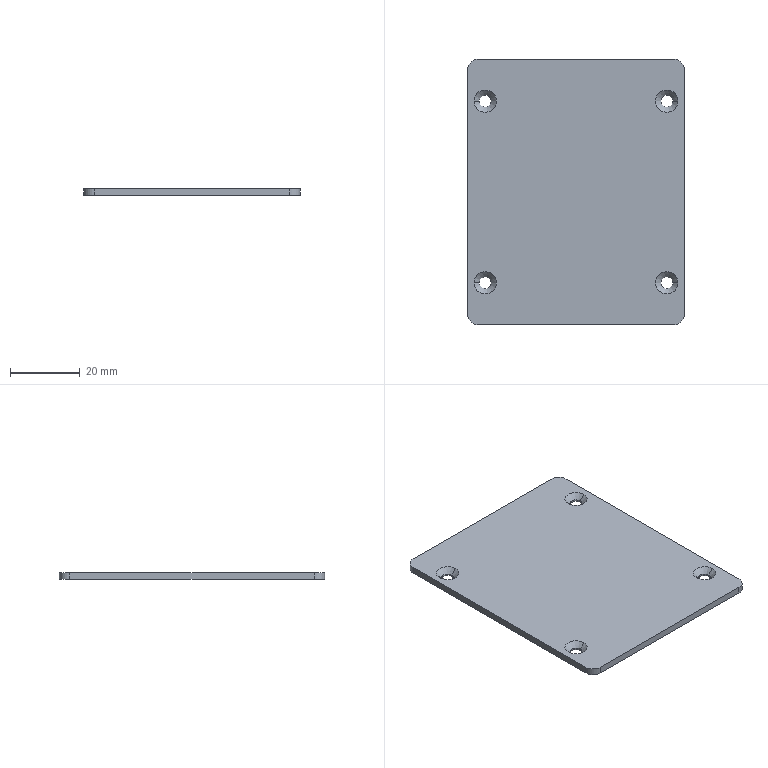Part | STEP file | 复件 FHB175-033^FHB175S-PRW-P40(马达RightUpper折-400W伺服电机) | 1 solid | 26 faces | box 62 x 76 x 2 mm | volume 9274 mm3 | cylinder 12 | cone 8 | plane 6 | commonest cylinder face diameters 3.4 x8 6 x4
STEP:
#1=CARTESIAN_POINT('',(-20.307,6.451,0.));
#2=VERTEX_POINT('',#1);
#3=CARTESIAN_POINT('',(-16.907,6.451,0.));
#4=VERTEX_POINT('',#3);
#5=CARTESIAN_POINT('',(-18.607,6.451,0.));
#6=DIRECTION('',(0.,0.,1.));
#7=DIRECTION('',(1.,0.,0.));
#8=AXIS2_PLACEMENT_3D('',#5,#6,#7);
#9=CIRCLE('',#8,1.7);
#10=EDGE_CURVE('',#2,#4,#9,.T.);
#11=ORIENTED_EDGE('',*,*,#10,.F.);
#12=CARTESIAN_POINT('',(-20.307,6.451,0.5));
#13=VERTEX_POINT('',#12);
#14=CARTESIAN_POINT('',(-20.307,6.451,2.));
#15=DIRECTION('',(0.,0.,1.));
#16=VECTOR('',#15,1000.);
#17=LINE('',#14,#16);
#18=EDGE_CURVE('',#2,#13,#17,.T.);
#19=ORIENTED_EDGE('',*,*,#18,.T.);
#20=CARTESIAN_POINT('',(-16.907,6.451,0.5));
#21=VERTEX_POINT('',#20);
#22=CARTESIAN_POINT('',(-18.607,6.451,0.5));
#23=DIRECTION('',(0.,0.,-1.));
#24=DIRECTION('',(1.,0.,0.));
#25=AXIS2_PLACEMENT_3D('',#22,#23,#24);
#26=CIRCLE('',#25,1.7);
#27=EDGE_CURVE('',#21,#13,#26,.T.);
#28=ORIENTED_EDGE('',*,*,#27,.F.);
#29=CARTESIAN_POINT('',(-16.907,6.451,2.));
#30=DIRECTION('',(0.,0.,1.));
#31=VECTOR('',#30,1000.);
#32=LINE('',#29,#31);
#33=EDGE_CURVE('',#4,#21,#32,.T.);
#34=ORIENTED_EDGE('',*,*,#33,.F.);
#35=EDGE_LOOP('',(#11,#19,#28,#34));
#36=FACE_OUTER_BOUND('',#35,.T.);
#37=CARTESIAN_POINT('',(-18.607,6.451,2.));
#38=DIRECTION('',(0.,0.,1.));
#39=DIRECTION('',(1.,0.,0.));
#40=AXIS2_PLACEMENT_3D('',#37,#38,#39);
#41=CYLINDRICAL_SURFACE('',#40,1.7);
#42=ADVANCED_FACE('',(#36),#41,.F.);
#43=CARTESIAN_POINT('',(-20.307,58.451,0.));
#44=VERTEX_POINT('',#43);
#45=CARTESIAN_POINT('',(-16.907,58.451,0.));
#46=VERTEX_POINT('',#45);
#47=CARTESIAN_POINT('',(-18.607,58.451,0.));
#48=DIRECTION('',(0.,0.,1.));
#49=DIRECTION('',(1.,0.,0.));
#50=AXIS2_PLACEMENT_3D('',#47,#48,#49);
#51=CIRCLE('',#50,1.7);
#52=EDGE_CURVE('',#44,#46,#51,.T.);
#53=ORIENTED_EDGE('',*,*,#52,.F.);
#54=CARTESIAN_POINT('',(-20.307,58.451,0.5));
#55=VERTEX_POINT('',#54);
#56=CARTESIAN_POINT('',(-20.307,58.451,2.));
#57=DIRECTION('',(0.,0.,1.));
#58=VECTOR('',#57,1000.);
#59=LINE('',#56,#58);
#60=EDGE_CURVE('',#44,#55,#59,.T.);
#61=ORIENTED_EDGE('',*,*,#60,.T.);
#62=CARTESIAN_POINT('',(-16.907,58.451,0.5));
#63=VERTEX_POINT('',#62);
#64=CARTESIAN_POINT('',(-18.607,58.451,0.5));
#65=DIRECTION('',(0.,0.,-1.));
#66=DIRECTION('',(1.,0.,0.));
#67=AXIS2_PLACEMENT_3D('',#64,#65,#66);
#68=CIRCLE('',#67,1.7);
#69=EDGE_CURVE('',#63,#55,#68,.T.);
#70=ORIENTED_EDGE('',*,*,#69,.F.);
#71=CARTESIAN_POINT('',(-16.907,58.451,2.));
#72=DIRECTION('',(0.,0.,1.));
#73=VECTOR('',#72,1000.);
#74=LINE('',#71,#73);
#75=EDGE_CURVE('',#46,#63,#74,.T.);
#76=ORIENTED_EDGE('',*,*,#75,.F.);
#77=EDGE_LOOP('',(#53,#61,#70,#76));
#78=FACE_OUTER_BOUND('',#77,.T.);
#79=CARTESIAN_POINT('',(-18.607,58.451,2.));
#80=DIRECTION('',(0.,0.,1.));
#81=DIRECTION('',(1.,0.,0.));
#82=AXIS2_PLACEMENT_3D('',#79,#80,#81);
#83=CYLINDRICAL_SURFACE('',#82,1.7);
#84=ADVANCED_FACE('',(#78),#83,.F.);
#85=CARTESIAN_POINT('',(31.693,58.451,0.));
#86=VERTEX_POINT('',#85);
#87=CARTESIAN_POINT('',(35.093,58.451,0.));
#88=VERTEX_POINT('',#87);
#89=CARTESIAN_POINT('',(33.393,58.451,0.));
#90=DIRECTION('',(0.,0.,1.));
#91=DIRECTION('',(1.,0.,0.));
#92=AXIS2_PLACEMENT_3D('',#89,#90,#91);
#93=CIRCLE('',#92,1.7);
#94=EDGE_CURVE('',#86,#88,#93,.T.);
#95=ORIENTED_EDGE('',*,*,#94,.F.);
#96=CARTESIAN_POINT('',(31.693,58.451,0.5));
#97=VERTEX_POINT('',#96);
#98=CARTESIAN_POINT('',(31.693,58.451,2.));
#99=DIRECTION('',(0.,0.,1.));
#100=VECTOR('',#99,1000.);
#101=LINE('',#98,#100);
#102=EDGE_CURVE('',#86,#97,#101,.T.);
#103=ORIENTED_EDGE('',*,*,#102,.T.);
#104=CARTESIAN_POINT('',(35.093,58.451,0.5));
#105=VERTEX_POINT('',#104);
#106=CARTESIAN_POINT('',(33.393,58.451,0.5));
#107=DIRECTION('',(0.,0.,-1.));
#108=DIRECTION('',(1.,0.,0.));
#109=AXIS2_PLACEMENT_3D('',#106,#107,#108);
#110=CIRCLE('',#109,1.7);
#111=EDGE_CURVE('',#105,#97,#110,.T.);
#112=ORIENTED_EDGE('',*,*,#111,.F.);
#113=CARTESIAN_POINT('',(35.093,58.451,2.));
#114=DIRECTION('',(0.,0.,1.));
#115=VECTOR('',#114,1000.);
#116=LINE('',#113,#115);
#117=EDGE_CURVE('',#88,#105,#116,.T.);
#118=ORIENTED_EDGE('',*,*,#117,.F.);
#119=EDGE_LOOP('',(#95,#103,#112,#118));
#120=FACE_OUTER_BOUND('',#119,.T.);
#121=CARTESIAN_POINT('',(33.393,58.451,2.));
#122=DIRECTION('',(0.,0.,1.));
#123=DIRECTION('',(1.,0.,0.));
#124=AXIS2_PLACEMENT_3D('',#121,#122,#123);
#125=CYLINDRICAL_SURFACE('',#124,1.7);
#126=ADVANCED_FACE('',(#120),#125,.F.);
#127=CARTESIAN_POINT('',(31.693,6.451,0.));
#128=VERTEX_POINT('',#127);
#129=CARTESIAN_POINT('',(35.093,6.451,0.));
#130=VERTEX_POINT('',#129);
#131=CARTESIAN_POINT('',(33.393,6.451,0.));
#132=DIRECTION('',(0.,0.,1.));
#133=DIRECTION('',(1.,0.,0.));
#134=AXIS2_PLACEMENT_3D('',#131,#132,#133);
#135=CIRCLE('',#134,1.7);
#136=EDGE_CURVE('',#128,#130,#135,.T.);
#137=ORIENTED_EDGE('',*,*,#136,.F.);
#138=CARTESIAN_POINT('',(31.693,6.451,0.5));
#139=VERTEX_POINT('',#138);
#140=CARTESIAN_POINT('',(31.693,6.451,2.));
#141=DIRECTION('',(0.,0.,1.));
#142=VECTOR('',#141,1000.);
#143=LINE('',#140,#142);
#144=EDGE_CURVE('',#128,#139,#143,.T.);
#145=ORIENTED_EDGE('',*,*,#144,.T.);
#146=CARTESIAN_POINT('',(35.093,6.451,0.5));
#147=VERTEX_POINT('',#146);
#148=CARTESIAN_POINT('',(33.393,6.451,0.5));
#149=DIRECTION('',(0.,0.,-1.));
#150=DIRECTION('',(1.,0.,0.));
#151=AXIS2_PLACEMENT_3D('',#148,#149,#150);
#152=CIRCLE('',#151,1.7);
#153=EDGE_CURVE('',#147,#139,#152,.T.);
#154=ORIENTED_EDGE('',*,*,#153,.F.);
#155=CARTESIAN_POINT('',(35.093,6.451,2.));
#156=DIRECTION('',(0.,0.,1.));
#157=VECTOR('',#156,1000.);
#158=LINE('',#155,#157);
#159=EDGE_CURVE('',#130,#147,#158,.T.);
#160=ORIENTED_EDGE('',*,*,#159,.F.);
#161=EDGE_LOOP('',(#137,#145,#154,#160));
#162=FACE_OUTER_BOUND('',#161,.T.);
#163=CARTESIAN_POINT('',(33.393,6.451,2.));
#164=DIRECTION('',(0.,0.,1.));
#165=DIRECTION('',(1.,0.,0.));
#166=AXIS2_PLACEMENT_3D('',#163,#164,#165);
#167=CYLINDRICAL_SURFACE('',#166,1.7);
#168=ADVANCED_FACE('',(#162),#167,.F.);
#169=ORIENTED_EDGE('',*,*,#27,.T.);
#170=CARTESIAN_POINT('',(-21.807,6.451,2.));
#171=VERTEX_POINT('',#170);
#172=CARTESIAN_POINT('',(-21.807,6.451,2.));
#173=DIRECTION('',(-0.7071,0.,0.7071));
#174=VECTOR('',#173,1000.);
#175=LINE('',#172,#174);
#176=EDGE_CURVE('',#13,#171,#175,.T.);
#177=ORIENTED_EDGE('',*,*,#176,.T.);
#178=CARTESIAN_POINT('',(-15.407,6.451,2.));
#179=VERTEX_POINT('',#178);
#180=CARTESIAN_POINT('',(-18.607,6.451,2.));
#181=DIRECTION('',(0.,0.,1.));
#182=DIRECTION('',(1.,0.,0.));
#183=AXIS2_PLACEMENT_3D('',#180,#181,#182);
#184=CIRCLE('',#183,3.2);
#185=EDGE_CURVE('',#171,#179,#184,.T.);
#186=ORIENTED_EDGE('',*,*,#185,.T.);
#187=CARTESIAN_POINT('',(-15.407,6.451,2.));
#188=DIRECTION('',(0.7071,0.,0.7071));
#189=VECTOR('',#188,1000.);
#190=LINE('',#187,#189);
#191=EDGE_CURVE('',#21,#179,#190,.T.);
#192=ORIENTED_EDGE('',*,*,#191,.F.);
#193=EDGE_LOOP('',(#169,#177,#186,#192));
#194=FACE_OUTER_BOUND('',#193,.T.);
#195=CARTESIAN_POINT('',(-18.607,6.451,2.));
#196=DIRECTION('',(0.,0.,1.));
#197=DIRECTION('',(1.,0.,0.));
#198=AXIS2_PLACEMENT_3D('',#195,#196,#197);
#199=CONICAL_SURFACE('',#198,3.2,0.7854);
#200=ADVANCED_FACE('',(#194),#199,.F.);
#201=ORIENTED_EDGE('',*,*,#69,.T.);
#202=CARTESIAN_POINT('',(-21.807,58.451,2.));
#203=VERTEX_POINT('',#202);
#204=CARTESIAN_POINT('',(-21.807,58.451,2.));
#205=DIRECTION('',(-0.7071,0.,0.7071));
#206=VECTOR('',#205,1000.);
#207=LINE('',#204,#206);
#208=EDGE_CURVE('',#55,#203,#207,.T.);
#209=ORIENTED_EDGE('',*,*,#208,.T.);
#210=CARTESIAN_POINT('',(-15.407,58.451,2.));
#211=VERTEX_POINT('',#210);
#212=CARTESIAN_POINT('',(-18.607,58.451,2.));
#213=DIRECTION('',(0.,0.,1.));
#214=DIRECTION('',(1.,0.,0.));
#215=AXIS2_PLACEMENT_3D('',#212,#213,#214);
#216=CIRCLE('',#215,3.2);
#217=EDGE_CURVE('',#203,#211,#216,.T.);
#218=ORIENTED_EDGE('',*,*,#217,.T.);
#219=CARTESIAN_POINT('',(-15.407,58.451,2.));
#220=DIRECTION('',(0.7071,0.,0.7071));
#221=VECTOR('',#220,1000.);
#222=LINE('',#219,#221);
#223=EDGE_CURVE('',#63,#211,#222,.T.);
#224=ORIENTED_EDGE('',*,*,#223,.F.);
#225=EDGE_LOOP('',(#201,#209,#218,#224));
#226=FACE_OUTER_BOUND('',#225,.T.);
#227=CARTESIAN_POINT('',(-18.607,58.451,2.));
#228=DIRECTION('',(0.,0.,1.));
#229=DIRECTION('',(1.,0.,0.));
#230=AXIS2_PLACEMENT_3D('',#227,#228,#229);
#231=CONICAL_SURFACE('',#230,3.2,0.7854);
#232=ADVANCED_FACE('',(#226),#231,.F.);
#233=ORIENTED_EDGE('',*,*,#111,.T.);
#234=CARTESIAN_POINT('',(30.193,58.451,2.));
#235=VERTEX_POINT('',#234);
#236=CARTESIAN_POINT('',(30.193,58.451,2.));
#237=DIRECTION('',(-0.7071,0.,0.7071));
#238=VECTOR('',#237,1000.);
#239=LINE('',#236,#238);
#240=EDGE_CURVE('',#97,#235,#239,.T.);
#241=ORIENTED_EDGE('',*,*,#240,.T.);
#242=CARTESIAN_POINT('',(36.593,58.451,2.));
#243=VERTEX_POINT('',#242);
#244=CARTESIAN_POINT('',(33.393,58.451,2.));
#245=DIRECTION('',(0.,0.,1.));
#246=DIRECTION('',(1.,0.,0.));
#247=AXIS2_PLACEMENT_3D('',#244,#245,#246);
#248=CIRCLE('',#247,3.2);
#249=EDGE_CURVE('',#235,#243,#248,.T.);
#250=ORIENTED_EDGE('',*,*,#249,.T.);
#251=CARTESIAN_POINT('',(36.593,58.451,2.));
#252=DIRECTION('',(0.7071,0.,0.7071));
#253=VECTOR('',#252,1000.);
#254=LINE('',#251,#253);
#255=EDGE_CURVE('',#105,#243,#254,.T.);
#256=ORIENTED_EDGE('',*,*,#255,.F.);
#257=EDGE_LOOP('',(#233,#241,#250,#256));
#258=FACE_OUTER_BOUND('',#257,.T.);
#259=CARTESIAN_POINT('',(33.393,58.451,2.));
#260=DIRECTION('',(0.,0.,1.));
#261=DIRECTION('',(1.,0.,0.));
#262=AXIS2_PLACEMENT_3D('',#259,#260,#261);
#263=CONICAL_SURFACE('',#262,3.2,0.7854);
#264=ADVANCED_FACE('',(#258),#263,.F.);
#265=ORIENTED_EDGE('',*,*,#153,.T.);
#266=CARTESIAN_POINT('',(30.193,6.451,2.));
#267=VERTEX_POINT('',#266);
#268=CARTESIAN_POINT('',(30.193,6.451,2.));
#269=DIRECTION('',(-0.7071,0.,0.7071));
#270=VECTOR('',#269,1000.);
#271=LINE('',#268,#270);
#272=EDGE_CURVE('',#139,#267,#271,.T.);
#273=ORIENTED_EDGE('',*,*,#272,.T.);
#274=CARTESIAN_POINT('',(36.593,6.451,2.));
#275=VERTEX_POINT('',#274);
#276=CARTESIAN_POINT('',(33.393,6.451,2.));
#277=DIRECTION('',(0.,0.,1.));
#278=DIRECTION('',(1.,0.,0.));
#279=AXIS2_PLACEMENT_3D('',#276,#277,#278);
#280=CIRCLE('',#279,3.2);
#281=EDGE_CURVE('',#267,#275,#280,.T.);
#282=ORIENTED_EDGE('',*,*,#281,.T.);
#283=CARTESIAN_POINT('',(36.593,6.451,2.));
#284=DIRECTION('',(0.7071,0.,0.7071));
#285=VECTOR('',#284,1000.);
#286=LINE('',#283,#285);
#287=EDGE_CURVE('',#147,#275,#286,.T.);
#288=ORIENTED_EDGE('',*,*,#287,.F.);
#289=EDGE_LOOP('',(#265,#273,#282,#288));
#290=FACE_OUTER_BOUND('',#289,.T.);
#291=CARTESIAN_POINT('',(33.393,6.451,2.));
#292=DIRECTION('',(0.,0.,1.));
#293=DIRECTION('',(1.,0.,0.));
#294=AXIS2_PLACEMENT_3D('',#291,#292,#293);
#295=CONICAL_SURFACE('',#294,3.2,0.7854);
#296=ADVANCED_FACE('',(#290),#295,.F.);
#297=CARTESIAN_POINT('',(38.393,67.451,0.));
#298=VERTEX_POINT('',#297);
#299=CARTESIAN_POINT('',(38.393,-2.549,0.));
#300=VERTEX_POINT('',#299);
#301=CARTESIAN_POINT('',(38.393,0.,0.));
#302=DIRECTION('',(0.,-1.,0.));
#303=VECTOR('',#302,1000.);
#304=LINE('',#301,#303);
#305=EDGE_CURVE('',#298,#300,#304,.T.);
#306=ORIENTED_EDGE('',*,*,#305,.T.);
#307=CARTESIAN_POINT('',(35.393,-5.549,0.));
#308=VERTEX_POINT('',#307);
#309=CARTESIAN_POINT('',(35.393,-2.549,0.));
#310=DIRECTION('',(0.,0.,-1.));
#311=DIRECTION('',(-1.,0.,0.));
#312=AXIS2_PLACEMENT_3D('',#309,#310,#311);
#313=CIRCLE('',#312,3.);
#314=EDGE_CURVE('',#300,#308,#313,.T.);
#315=ORIENTED_EDGE('',*,*,#314,.T.);
#316=CARTESIAN_POINT('',(-20.607,-5.549,0.));
#317=VERTEX_POINT('',#316);
#318=CARTESIAN_POINT('',(0.,-5.549,0.));
#319=DIRECTION('',(-1.,0.,0.));
#320=VECTOR('',#319,1000.);
#321=LINE('',#318,#320);
#322=EDGE_CURVE('',#308,#317,#321,.T.);
#323=ORIENTED_EDGE('',*,*,#322,.T.);
#324=CARTESIAN_POINT('',(-23.607,-2.549,0.));
#325=VERTEX_POINT('',#324);
#326=CARTESIAN_POINT('',(-20.607,-2.549,0.));
#327=DIRECTION('',(0.,0.,-1.));
#328=DIRECTION('',(-1.,0.,0.));
#329=AXIS2_PLACEMENT_3D('',#326,#327,#328);
#330=CIRCLE('',#329,3.);
#331=EDGE_CURVE('',#317,#325,#330,.T.);
#332=ORIENTED_EDGE('',*,*,#331,.T.);
#333=CARTESIAN_POINT('',(-23.607,67.451,0.));
#334=VERTEX_POINT('',#333);
#335=CARTESIAN_POINT('',(-23.607,0.,0.));
#336=DIRECTION('',(0.,1.,0.));
#337=VECTOR('',#336,1000.);
#338=LINE('',#335,#337);
#339=EDGE_CURVE('',#325,#334,#338,.T.);
#340=ORIENTED_EDGE('',*,*,#339,.T.);
#341=CARTESIAN_POINT('',(-20.607,70.451,0.));
#342=VERTEX_POINT('',#341);
#343=CARTESIAN_POINT('',(-20.607,67.451,0.));
#344=DIRECTION('',(0.,0.,-1.));
#345=DIRECTION('',(-1.,0.,0.));
#346=AXIS2_PLACEMENT_3D('',#343,#344,#345);
#347=CIRCLE('',#346,3.);
#348=EDGE_CURVE('',#334,#342,#347,.T.);
#349=ORIENTED_EDGE('',*,*,#348,.T.);
#350=CARTESIAN_POINT('',(35.393,70.451,0.));
#351=VERTEX_POINT('',#350);
#352=CARTESIAN_POINT('',(0.,70.451,0.));
#353=DIRECTION('',(1.,0.,0.));
#354=VECTOR('',#353,1000.);
#355=LINE('',#352,#354);
#356=EDGE_CURVE('',#342,#351,#355,.T.);
#357=ORIENTED_EDGE('',*,*,#356,.T.);
#358=CARTESIAN_POINT('',(35.393,67.451,0.));
#359=DIRECTION('',(0.,0.,-1.));
#360=DIRECTION('',(-1.,0.,0.));
#361=AXIS2_PLACEMENT_3D('',#358,#359,#360);
#362=CIRCLE('',#361,3.);
#363=EDGE_CURVE('',#351,#298,#362,.T.);
#364=ORIENTED_EDGE('',*,*,#363,.T.);
#365=EDGE_LOOP('',(#306,#315,#323,#332,#340,#349,#357,#364));
#366=FACE_OUTER_BOUND('',#365,.T.);
#367=CARTESIAN_POINT('',(-18.607,6.451,0.));
#368=DIRECTION('',(0.,0.,1.));
#369=DIRECTION('',(1.,0.,0.));
#370=AXIS2_PLACEMENT_3D('',#367,#368,#369);
#371=CIRCLE('',#370,1.7);
#372=EDGE_CURVE('',#4,#2,#371,.T.);
#373=ORIENTED_EDGE('',*,*,#372,.T.);
#374=ORIENTED_EDGE('',*,*,#10,.T.);
#375=EDGE_LOOP('',(#373,#374));
#376=FACE_BOUND('',#375,.T.);
#377=CARTESIAN_POINT('',(-18.607,58.451,0.));
#378=DIRECTION('',(0.,0.,1.));
#379=DIRECTION('',(1.,0.,0.));
#380=AXIS2_PLACEMENT_3D('',#377,#378,#379);
#381=CIRCLE('',#380,1.7);
#382=EDGE_CURVE('',#46,#44,#381,.T.);
#383=ORIENTED_EDGE('',*,*,#382,.T.);
#384=ORIENTED_EDGE('',*,*,#52,.T.);
#385=EDGE_LOOP('',(#383,#384));
#386=FACE_BOUND('',#385,.T.);
#387=CARTESIAN_POINT('',(33.393,58.451,0.));
#388=DIRECTION('',(0.,0.,1.));
#389=DIRECTION('',(1.,0.,0.));
#390=AXIS2_PLACEMENT_3D('',#387,#388,#389);
#391=CIRCLE('',#390,1.7);
#392=EDGE_CURVE('',#88,#86,#391,.T.);
#393=ORIENTED_EDGE('',*,*,#392,.T.);
#394=ORIENTED_EDGE('',*,*,#94,.T.);
#395=EDGE_LOOP('',(#393,#394));
#396=FACE_BOUND('',#395,.T.);
#397=CARTESIAN_POINT('',(33.393,6.451,0.));
#398=DIRECTION('',(0.,0.,1.));
#399=DIRECTION('',(1.,0.,0.));
#400=AXIS2_PLACEMENT_3D('',#397,#398,#399);
#401=CIRCLE('',#400,1.7);
#402=EDGE_CURVE('',#130,#128,#401,.T.);
#403=ORIENTED_EDGE('',*,*,#402,.T.);
#404=ORIENTED_EDGE('',*,*,#136,.T.);
#405=EDGE_LOOP('',(#403,#404));
#406=FACE_BOUND('',#405,.T.);
#407=CARTESIAN_POINT('',(0.,0.,0.));
#408=DIRECTION('',(0.,0.,-1.));
#409=DIRECTION('',(-1.,0.,0.));
#410=AXIS2_PLACEMENT_3D('',#407,#408,#409);
#411=PLANE('',#410);
#412=ADVANCED_FACE('',(#366,#376,#386,#396,#406),#411,.T.);
#413=ORIENTED_EDGE('',*,*,#314,.F.);
#414=CARTESIAN_POINT('',(38.393,-2.549,2.));
#415=VERTEX_POINT('',#414);
#416=CARTESIAN_POINT('',(38.393,-2.549,2.));
#417=DIRECTION('',(0.,0.,1.));
#418=VECTOR('',#417,1000.);
#419=LINE('',#416,#418);
#420=EDGE_CURVE('',#300,#415,#419,.T.);
#421=ORIENTED_EDGE('',*,*,#420,.T.);
#422=CARTESIAN_POINT('',(35.393,-5.549,2.));
#423=VERTEX_POINT('',#422);
#424=CARTESIAN_POINT('',(35.393,-2.549,2.));
#425=DIRECTION('',(0.,0.,-1.));
#426=DIRECTION('',(-1.,0.,0.));
#427=AXIS2_PLACEMENT_3D('',#424,#425,#426);
#428=CIRCLE('',#427,3.);
#429=EDGE_CURVE('',#415,#423,#428,.T.);
#430=ORIENTED_EDGE('',*,*,#429,.T.);
#431=CARTESIAN_POINT('',(35.393,-5.549,2.));
#432=DIRECTION('',(0.,0.,-1.));
#433=VECTOR('',#432,1000.);
#434=LINE('',#431,#433);
#435=EDGE_CURVE('',#423,#308,#434,.T.);
#436=ORIENTED_EDGE('',*,*,#435,.T.);
#437=EDGE_LOOP('',(#413,#421,#430,#436));
#438=FACE_OUTER_BOUND('',#437,.T.);
#439=CARTESIAN_POINT('',(35.393,-2.549,2.));
#440=DIRECTION('',(0.,0.,-1.));
#441=DIRECTION('',(-1.,0.,0.));
#442=AXIS2_PLACEMENT_3D('',#439,#440,#441);
#443=CYLINDRICAL_SURFACE('',#442,3.);
#444=ADVANCED_FACE('',(#438),#443,.T.);
#445=ORIENTED_EDGE('',*,*,#420,.F.);
#446=ORIENTED_EDGE('',*,*,#305,.F.);
#447=CARTESIAN_POINT('',(38.393,67.451,2.));
#448=VERTEX_POINT('',#447);
#449=CARTESIAN_POINT('',(38.393,67.451,2.));
#450=DIRECTION('',(0.,0.,-1.));
#451=VECTOR('',#450,1000.);
#452=LINE('',#449,#451);
#453=EDGE_CURVE('',#448,#298,#452,.T.);
#454=ORIENTED_EDGE('',*,*,#453,.F.);
#455=CARTESIAN_POINT('',(38.393,-5.549,2.));
#456=DIRECTION('',(0.,1.,0.));
#457=VECTOR('',#456,1000.);
#458=LINE('',#455,#457);
#459=EDGE_CURVE('',#415,#448,#458,.T.);
#460=ORIENTED_EDGE('',*,*,#459,.F.);
#461=EDGE_LOOP('',(#445,#446,#454,#460));
#462=FACE_OUTER_BOUND('',#461,.T.);
#463=CARTESIAN_POINT('',(38.393,-5.549,2.));
#464=DIRECTION('',(-1.,0.,0.));
#465=DIRECTION('',(0.,0.,1.));
#466=AXIS2_PLACEMENT_3D('',#463,#464,#465);
#467=PLANE('',#466);
#468=ADVANCED_FACE('',(#462),#467,.F.);
#469=ORIENTED_EDGE('',*,*,#363,.F.);
#470=CARTESIAN_POINT('',(35.393,70.451,2.));
#471=VERTEX_POINT('',#470);
#472=CARTESIAN_POINT('',(35.393,70.451,2.));
#473=DIRECTION('',(0.,0.,1.));
#474=VECTOR('',#473,1000.);
#475=LINE('',#472,#474);
#476=EDGE_CURVE('',#351,#471,#475,.T.);
#477=ORIENTED_EDGE('',*,*,#476,.T.);
#478=CARTESIAN_POINT('',(35.393,67.451,2.));
#479=DIRECTION('',(0.,0.,-1.));
#480=DIRECTION('',(-1.,0.,0.));
#481=AXIS2_PLACEMENT_3D('',#478,#479,#480);
#482=CIRCLE('',#481,3.);
#483=EDGE_CURVE('',#471,#448,#482,.T.);
#484=ORIENTED_EDGE('',*,*,#483,.T.);
#485=ORIENTED_EDGE('',*,*,#453,.T.);
#486=EDGE_LOOP('',(#469,#477,#484,#485));
#487=FACE_OUTER_BOUND('',#486,.T.);
#488=CARTESIAN_POINT('',(35.393,67.451,2.));
#489=DIRECTION('',(0.,0.,-1.));
#490=DIRECTION('',(-1.,0.,0.));
#491=AXIS2_PLACEMENT_3D('',#488,#489,#490);
#492=CYLINDRICAL_SURFACE('',#491,3.);
#493=ADVANCED_FACE('',(#487),#492,.T.);
#494=CARTESIAN_POINT('',(-20.607,70.451,2.));
#495=VERTEX_POINT('',#494);
#496=CARTESIAN_POINT('',(-20.607,70.451,2.));
#497=DIRECTION('',(0.,0.,-1.));
#498=VECTOR('',#497,1000.);
#499=LINE('',#496,#498);
#500=EDGE_CURVE('',#495,#342,#499,.T.);
#501=ORIENTED_EDGE('',*,*,#500,.F.);
#502=CARTESIAN_POINT('',(-23.607,70.451,2.));
#503=DIRECTION('',(-1.,0.,0.));
#504=VECTOR('',#503,1000.);
#505=LINE('',#502,#504);
#506=EDGE_CURVE('',#471,#495,#505,.T.);
#507=ORIENTED_EDGE('',*,*,#506,.F.);
#508=ORIENTED_EDGE('',*,*,#476,.F.);
#509=ORIENTED_EDGE('',*,*,#356,.F.);
#510=EDGE_LOOP('',(#501,#507,#508,#509));
#511=FACE_OUTER_BOUND('',#510,.T.);
#512=CARTESIAN_POINT('',(-23.607,70.451,2.));
#513=DIRECTION('',(0.,-1.,0.));
#514=DIRECTION('',(0.,0.,-1.));
#515=AXIS2_PLACEMENT_3D('',#512,#513,#514);
#516=PLANE('',#515);
#517=ADVANCED_FACE('',(#511),#516,.F.);
#518=ORIENTED_EDGE('',*,*,#348,.F.);
#519=CARTESIAN_POINT('',(-23.607,67.451,2.));
#520=VERTEX_POINT('',#519);
#521=CARTESIAN_POINT('',(-23.607,67.451,2.));
#522=DIRECTION('',(0.,0.,1.));
#523=VECTOR('',#522,1000.);
#524=LINE('',#521,#523);
#525=EDGE_CURVE('',#334,#520,#524,.T.);
#526=ORIENTED_EDGE('',*,*,#525,.T.);
#527=CARTESIAN_POINT('',(-20.607,67.451,2.));
#528=DIRECTION('',(0.,0.,-1.));
#529=DIRECTION('',(-1.,0.,0.));
#530=AXIS2_PLACEMENT_3D('',#527,#528,#529);
#531=CIRCLE('',#530,3.);
#532=EDGE_CURVE('',#520,#495,#531,.T.);
#533=ORIENTED_EDGE('',*,*,#532,.T.);
#534=ORIENTED_EDGE('',*,*,#500,.T.);
#535=EDGE_LOOP('',(#518,#526,#533,#534));
#536=FACE_OUTER_BOUND('',#535,.T.);
#537=CARTESIAN_POINT('',(-20.607,67.451,2.));
#538=DIRECTION('',(0.,0.,-1.));
#539=DIRECTION('',(-1.,0.,0.));
#540=AXIS2_PLACEMENT_3D('',#537,#538,#539);
#541=CYLINDRICAL_SURFACE('',#540,3.);
#542=ADVANCED_FACE('',(#536),#541,.T.);
#543=CARTESIAN_POINT('',(-23.607,-2.549,2.));
#544=VERTEX_POINT('',#543);
#545=CARTESIAN_POINT('',(-23.607,-2.549,2.));
#546=DIRECTION('',(0.,0.,-1.));
#547=VECTOR('',#546,1000.);
#548=LINE('',#545,#547);
#549=EDGE_CURVE('',#544,#325,#548,.T.);
#550=ORIENTED_EDGE('',*,*,#549,.F.);
#551=CARTESIAN_POINT('',(-23.607,-5.549,2.));
#552=DIRECTION('',(0.,-1.,0.));
#553=VECTOR('',#552,1000.);
#554=LINE('',#551,#553);
#555=EDGE_CURVE('',#520,#544,#554,.T.);
#556=ORIENTED_EDGE('',*,*,#555,.F.);
#557=ORIENTED_EDGE('',*,*,#525,.F.);
#558=ORIENTED_EDGE('',*,*,#339,.F.);
#559=EDGE_LOOP('',(#550,#556,#557,#558));
#560=FACE_OUTER_BOUND('',#559,.T.);
#561=CARTESIAN_POINT('',(-23.607,-5.549,2.));
#562=DIRECTION('',(1.,0.,0.));
#563=DIRECTION('',(0.,0.,-1.));
#564=AXIS2_PLACEMENT_3D('',#561,#562,#563);
#565=PLANE('',#564);
#566=ADVANCED_FACE('',(#560),#565,.F.);
#567=ORIENTED_EDGE('',*,*,#331,.F.);
#568=CARTESIAN_POINT('',(-20.607,-5.549,2.));
#569=VERTEX_POINT('',#568);
#570=CARTESIAN_POINT('',(-20.607,-5.549,2.));
#571=DIRECTION('',(0.,0.,1.));
#572=VECTOR('',#571,1000.);
#573=LINE('',#570,#572);
#574=EDGE_CURVE('',#317,#569,#573,.T.);
#575=ORIENTED_EDGE('',*,*,#574,.T.);
#576=CARTESIAN_POINT('',(-20.607,-2.549,2.));
#577=DIRECTION('',(0.,0.,-1.));
#578=DIRECTION('',(-1.,0.,0.));
#579=AXIS2_PLACEMENT_3D('',#576,#577,#578);
#580=CIRCLE('',#579,3.);
#581=EDGE_CURVE('',#569,#544,#580,.T.);
#582=ORIENTED_EDGE('',*,*,#581,.T.);
#583=ORIENTED_EDGE('',*,*,#549,.T.);
#584=EDGE_LOOP('',(#567,#575,#582,#583));
#585=FACE_OUTER_BOUND('',#584,.T.);
#586=CARTESIAN_POINT('',(-20.607,-2.549,2.));
#587=DIRECTION('',(0.,0.,-1.));
#588=DIRECTION('',(-1.,0.,0.));
#589=AXIS2_PLACEMENT_3D('',#586,#587,#588);
#590=CYLINDRICAL_SURFACE('',#589,3.);
#591=ADVANCED_FACE('',(#585),#590,.T.);
#592=ORIENTED_EDGE('',*,*,#574,.F.);
#593=ORIENTED_EDGE('',*,*,#322,.F.);
#594=ORIENTED_EDGE('',*,*,#435,.F.);
#595=CARTESIAN_POINT('',(-23.607,-5.549,2.));
#596=DIRECTION('',(1.,0.,0.));
#597=VECTOR('',#596,1000.);
#598=LINE('',#595,#597);
#599=EDGE_CURVE('',#569,#423,#598,.T.);
#600=ORIENTED_EDGE('',*,*,#599,.F.);
#601=EDGE_LOOP('',(#592,#593,#594,#600));
#602=FACE_OUTER_BOUND('',#601,.T.);
#603=CARTESIAN_POINT('',(-23.607,-5.549,2.));
#604=DIRECTION('',(0.,1.,0.));
#605=DIRECTION('',(0.,0.,1.));
#606=AXIS2_PLACEMENT_3D('',#603,#604,#605);
#607=PLANE('',#606);
#608=ADVANCED_FACE('',(#602),#607,.F.);
#609=ORIENTED_EDGE('',*,*,#18,.F.);
#610=ORIENTED_EDGE('',*,*,#372,.F.);
#611=ORIENTED_EDGE('',*,*,#33,.T.);
#612=CARTESIAN_POINT('',(-18.607,6.451,0.5));
#613=DIRECTION('',(0.,0.,-1.));
#614=DIRECTION('',(1.,0.,0.));
#615=AXIS2_PLACEMENT_3D('',#612,#613,#614);
#616=CIRCLE('',#615,1.7);
#617=EDGE_CURVE('',#13,#21,#616,.T.);
#618=ORIENTED_EDGE('',*,*,#617,.F.);
#619=EDGE_LOOP('',(#609,#610,#611,#618));
#620=FACE_OUTER_BOUND('',#619,.T.);
#621=CARTESIAN_POINT('',(-18.607,6.451,2.));
#622=DIRECTION('',(0.,0.,1.));
#623=DIRECTION('',(1.,0.,0.));
#624=AXIS2_PLACEMENT_3D('',#621,#622,#623);
#625=CYLINDRICAL_SURFACE('',#624,1.7);
#626=ADVANCED_FACE('',(#620),#625,.F.);
#627=ORIENTED_EDGE('',*,*,#60,.F.);
#628=ORIENTED_EDGE('',*,*,#382,.F.);
#629=ORIENTED_EDGE('',*,*,#75,.T.);
#630=CARTESIAN_POINT('',(-18.607,58.451,0.5));
#631=DIRECTION('',(0.,0.,-1.));
#632=DIRECTION('',(1.,0.,0.));
#633=AXIS2_PLACEMENT_3D('',#630,#631,#632);
#634=CIRCLE('',#633,1.7);
#635=EDGE_CURVE('',#55,#63,#634,.T.);
#636=ORIENTED_EDGE('',*,*,#635,.F.);
#637=EDGE_LOOP('',(#627,#628,#629,#636));
#638=FACE_OUTER_BOUND('',#637,.T.);
#639=CARTESIAN_POINT('',(-18.607,58.451,2.));
#640=DIRECTION('',(0.,0.,1.));
#641=DIRECTION('',(1.,0.,0.));
#642=AXIS2_PLACEMENT_3D('',#639,#640,#641);
#643=CYLINDRICAL_SURFACE('',#642,1.7);
#644=ADVANCED_FACE('',(#638),#643,.F.);
#645=ORIENTED_EDGE('',*,*,#102,.F.);
#646=ORIENTED_EDGE('',*,*,#392,.F.);
#647=ORIENTED_EDGE('',*,*,#117,.T.);
#648=CARTESIAN_POINT('',(33.393,58.451,0.5));
#649=DIRECTION('',(0.,0.,-1.));
#650=DIRECTION('',(1.,0.,0.));
#651=AXIS2_PLACEMENT_3D('',#648,#649,#650);
#652=CIRCLE('',#651,1.7);
#653=EDGE_CURVE('',#97,#105,#652,.T.);
#654=ORIENTED_EDGE('',*,*,#653,.F.);
#655=EDGE_LOOP('',(#645,#646,#647,#654));
#656=FACE_OUTER_BOUND('',#655,.T.);
#657=CARTESIAN_POINT('',(33.393,58.451,2.));
#658=DIRECTION('',(0.,0.,1.));
#659=DIRECTION('',(1.,0.,0.));
#660=AXIS2_PLACEMENT_3D('',#657,#658,#659);
#661=CYLINDRICAL_SURFACE('',#660,1.7);
#662=ADVANCED_FACE('',(#656),#661,.F.);
#663=ORIENTED_EDGE('',*,*,#144,.F.);
#664=ORIENTED_EDGE('',*,*,#402,.F.);
#665=ORIENTED_EDGE('',*,*,#159,.T.);
#666=CARTESIAN_POINT('',(33.393,6.451,0.5));
#667=DIRECTION('',(0.,0.,-1.));
#668=DIRECTION('',(1.,0.,0.));
#669=AXIS2_PLACEMENT_3D('',#666,#667,#668);
#670=CIRCLE('',#669,1.7);
#671=EDGE_CURVE('',#139,#147,#670,.T.);
#672=ORIENTED_EDGE('',*,*,#671,.F.);
#673=EDGE_LOOP('',(#663,#664,#665,#672));
#674=FACE_OUTER_BOUND('',#673,.T.);
#675=CARTESIAN_POINT('',(33.393,6.451,2.));
#676=DIRECTION('',(0.,0.,1.));
#677=DIRECTION('',(1.,0.,0.));
#678=AXIS2_PLACEMENT_3D('',#675,#676,#677);
#679=CYLINDRICAL_SURFACE('',#678,1.7);
#680=ADVANCED_FACE('',(#674),#679,.F.);
#681=ORIENTED_EDGE('',*,*,#581,.F.);
#682=ORIENTED_EDGE('',*,*,#599,.T.);
#683=ORIENTED_EDGE('',*,*,#429,.F.);
#684=ORIENTED_EDGE('',*,*,#459,.T.);
#685=ORIENTED_EDGE('',*,*,#483,.F.);
#686=ORIENTED_EDGE('',*,*,#506,.T.);
#687=ORIENTED_EDGE('',*,*,#532,.F.);
#688=ORIENTED_EDGE('',*,*,#555,.T.);
#689=EDGE_LOOP('',(#681,#682,#683,#684,#685,#686,#687,#688));
#690=FACE_OUTER_BOUND('',#689,.T.);
#691=CARTESIAN_POINT('',(-18.607,6.451,2.));
#692=DIRECTION('',(0.,0.,1.));
#693=DIRECTION('',(1.,0.,0.));
#694=AXIS2_PLACEMENT_3D('',#691,#692,#693);
#695=CIRCLE('',#694,3.2);
#696=EDGE_CURVE('',#179,#171,#695,.T.);
#697=ORIENTED_EDGE('',*,*,#696,.F.);
#698=ORIENTED_EDGE('',*,*,#185,.F.);
#699=EDGE_LOOP('',(#697,#698));
#700=FACE_BOUND('',#699,.T.);
#701=CARTESIAN_POINT('',(-18.607,58.451,2.));
#702=DIRECTION('',(0.,0.,1.));
#703=DIRECTION('',(1.,0.,0.));
#704=AXIS2_PLACEMENT_3D('',#701,#702,#703);
#705=CIRCLE('',#704,3.2);
#706=EDGE_CURVE('',#211,#203,#705,.T.);
#707=ORIENTED_EDGE('',*,*,#706,.F.);
#708=ORIENTED_EDGE('',*,*,#217,.F.);
#709=EDGE_LOOP('',(#707,#708));
#710=FACE_BOUND('',#709,.T.);
#711=CARTESIAN_POINT('',(33.393,58.451,2.));
#712=DIRECTION('',(0.,0.,1.));
#713=DIRECTION('',(1.,0.,0.));
#714=AXIS2_PLACEMENT_3D('',#711,#712,#713);
#715=CIRCLE('',#714,3.2);
#716=EDGE_CURVE('',#243,#235,#715,.T.);
#717=ORIENTED_EDGE('',*,*,#716,.F.);
#718=ORIENTED_EDGE('',*,*,#249,.F.);
#719=EDGE_LOOP('',(#717,#718));
#720=FACE_BOUND('',#719,.T.);
#721=CARTESIAN_POINT('',(33.393,6.451,2.));
#722=DIRECTION('',(0.,0.,1.));
#723=DIRECTION('',(1.,0.,0.));
#724=AXIS2_PLACEMENT_3D('',#721,#722,#723);
#725=CIRCLE('',#724,3.2);
#726=EDGE_CURVE('',#275,#267,#725,.T.);
#727=ORIENTED_EDGE('',*,*,#726,.F.);
#728=ORIENTED_EDGE('',*,*,#281,.F.);
#729=EDGE_LOOP('',(#727,#728));
#730=FACE_BOUND('',#729,.T.);
#731=CARTESIAN_POINT('',(0.,0.,2.));
#732=DIRECTION('',(0.,0.,-1.));
#733=DIRECTION('',(-1.,0.,0.));
#734=AXIS2_PLACEMENT_3D('',#731,#732,#733);
#735=PLANE('',#734);
#736=ADVANCED_FACE('',(#690,#700,#710,#720,#730),#735,.F.);
#737=ORIENTED_EDGE('',*,*,#176,.F.);
#738=ORIENTED_EDGE('',*,*,#617,.T.);
#739=ORIENTED_EDGE('',*,*,#191,.T.);
#740=ORIENTED_EDGE('',*,*,#696,.T.);
#741=EDGE_LOOP('',(#737,#738,#739,#740));
#742=FACE_OUTER_BOUND('',#741,.T.);
#743=CARTESIAN_POINT('',(-18.607,6.451,2.));
#744=DIRECTION('',(0.,0.,1.));
#745=DIRECTION('',(1.,0.,0.));
#746=AXIS2_PLACEMENT_3D('',#743,#744,#745);
#747=CONICAL_SURFACE('',#746,3.2,0.7854);
#748=ADVANCED_FACE('',(#742),#747,.F.);
#749=ORIENTED_EDGE('',*,*,#208,.F.);
#750=ORIENTED_EDGE('',*,*,#635,.T.);
#751=ORIENTED_EDGE('',*,*,#223,.T.);
#752=ORIENTED_EDGE('',*,*,#706,.T.);
#753=EDGE_LOOP('',(#749,#750,#751,#752));
#754=FACE_OUTER_BOUND('',#753,.T.);
#755=CARTESIAN_POINT('',(-18.607,58.451,2.));
#756=DIRECTION('',(0.,0.,1.));
#757=DIRECTION('',(1.,0.,0.));
#758=AXIS2_PLACEMENT_3D('',#755,#756,#757);
#759=CONICAL_SURFACE('',#758,3.2,0.7854);
#760=ADVANCED_FACE('',(#754),#759,.F.);
#761=ORIENTED_EDGE('',*,*,#240,.F.);
#762=ORIENTED_EDGE('',*,*,#653,.T.);
#763=ORIENTED_EDGE('',*,*,#255,.T.);
#764=ORIENTED_EDGE('',*,*,#716,.T.);
#765=EDGE_LOOP('',(#761,#762,#763,#764));
#766=FACE_OUTER_BOUND('',#765,.T.);
#767=CARTESIAN_POINT('',(33.393,58.451,2.));
#768=DIRECTION('',(0.,0.,1.));
#769=DIRECTION('',(1.,0.,0.));
#770=AXIS2_PLACEMENT_3D('',#767,#768,#769);
#771=CONICAL_SURFACE('',#770,3.2,0.7854);
#772=ADVANCED_FACE('',(#766),#771,.F.);
#773=ORIENTED_EDGE('',*,*,#272,.F.);
#774=ORIENTED_EDGE('',*,*,#671,.T.);
#775=ORIENTED_EDGE('',*,*,#287,.T.);
#776=ORIENTED_EDGE('',*,*,#726,.T.);
#777=EDGE_LOOP('',(#773,#774,#775,#776));
#778=FACE_OUTER_BOUND('',#777,.T.);
#779=CARTESIAN_POINT('',(33.393,6.451,2.));
#780=DIRECTION('',(0.,0.,1.));
#781=DIRECTION('',(1.,0.,0.));
#782=AXIS2_PLACEMENT_3D('',#779,#780,#781);
#783=CONICAL_SURFACE('',#782,3.2,0.7854);
#784=ADVANCED_FACE('',(#778),#783,.F.);
#785=CLOSED_SHELL('',(#42,#84,#126,#168,#200,#232,#264,#296,#412,#444,#468,#493,#517,#542,#566,#591,#608,#626,#644,#662,#680,#736,#748,#760,#772,#784));
#786=MANIFOLD_SOLID_BREP('',#785);
#787=CARTESIAN_POINT('',(0.,0.,0.));
#788=DIRECTION('',(0.,0.,1.));
#789=DIRECTION('',(1.,0.,0.));
#790=AXIS2_PLACEMENT_3D('',#787,#788,#789);
#791=(LENGTH_UNIT()NAMED_UNIT(*)SI_UNIT(.MILLI.,.METRE.));
#792=UNCERTAINTY_MEASURE_WITH_UNIT(LENGTH_MEASURE(0.00001),#791,'','');
#793=(NAMED_UNIT(*)PLANE_ANGLE_UNIT()SI_UNIT($,.RADIAN.));
#794=(NAMED_UNIT(*)SI_UNIT($,.STERADIAN.)SOLID_ANGLE_UNIT());
#795=(GEOMETRIC_REPRESENTATION_CONTEXT(3)GLOBAL_UNCERTAINTY_ASSIGNED_CONTEXT((#792))GLOBAL_UNIT_ASSIGNED_CONTEXT((#791,#793,#794))REPRESENTATION_CONTEXT('',''));
#796=ADVANCED_BREP_SHAPE_REPRESENTATION('',(#786,#790),#795);